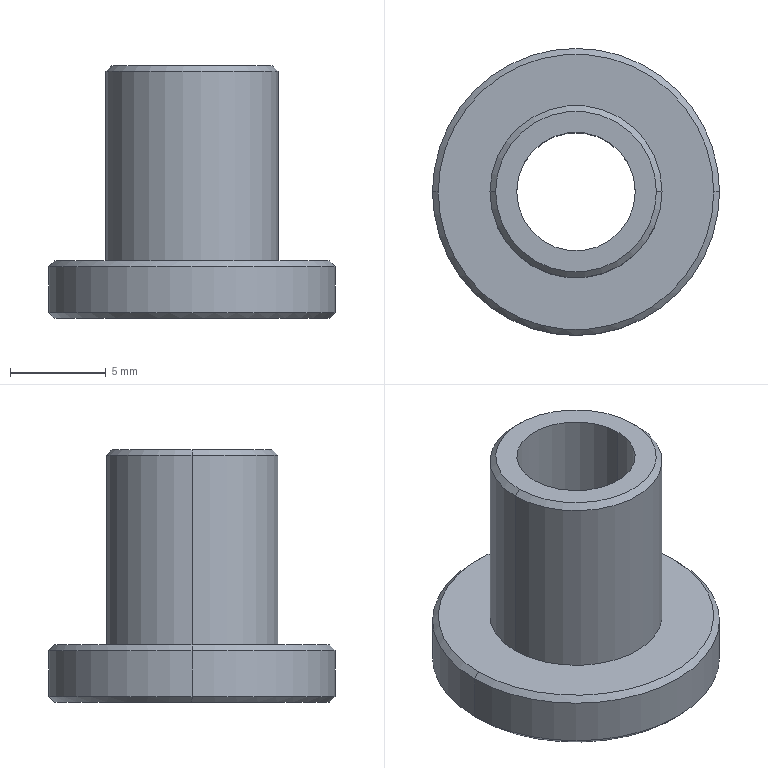Part | STEP file | 1 solid | 15 faces | box 15 x 15 x 13.2 mm | volume 775.094 mm3 | cone 6 | cylinder 6 | plane 3 | commonest cylinder face diameters 6.2 x2 9 x2 15 x2
STEP:
#1=CARTESIAN_POINT('',(0.,0.,0.));
#2=DIRECTION('',(0.,0.,1.));
#3=DIRECTION('',(1.,0.,0.));
#4=AXIS2_PLACEMENT_3D('',#1,#2,#3);
#5=CARTESIAN_POINT('',(-7.2,0.,0.));
#6=VERTEX_POINT('',#5);
#7=CARTESIAN_POINT('',(7.2,0.,0.));
#8=VERTEX_POINT('',#7);
#9=CARTESIAN_POINT('',(0.,0.,0.));
#10=DIRECTION('',(0.,0.,-1.));
#11=DIRECTION('',(1.,0.,0.));
#12=AXIS2_PLACEMENT_3D('',#9,#10,#11);
#13=CIRCLE('',#12,7.2);
#14=CARTESIAN_POINT('',(0.,0.,0.));
#15=DIRECTION('',(0.,0.,1.));
#16=DIRECTION('',(1.,0.,0.));
#17=AXIS2_PLACEMENT_3D('',#14,#15,#16);
#18=CONICAL_SURFACE('',#17,7.2,0.7854);
#19=CARTESIAN_POINT('',(6.283,0.));
#20=DIRECTION('',(-1.,0.));
#21=VECTOR('',#20,1.);
#22=LINE('',#19,#21);
#23=(GEOMETRIC_REPRESENTATION_CONTEXT(2)PARAMETRIC_REPRESENTATION_CONTEXT()REPRESENTATION_CONTEXT('',''));
#24=DEFINITIONAL_REPRESENTATION('',(#22),#23);
#25=PCURVE('',#18,#24);
#26=CARTESIAN_POINT('',(0.,0.,0.));
#27=DIRECTION('',(0.,0.,1.));
#28=DIRECTION('',(1.,0.,0.));
#29=AXIS2_PLACEMENT_3D('',#26,#27,#28);
#30=PLANE('',#29);
#31=CARTESIAN_POINT('',(7.2,0.));
#32=CARTESIAN_POINT('',(7.2,-12.471));
#33=CARTESIAN_POINT('',(-3.6,-6.235));
#34=CARTESIAN_POINT('',(-14.4,0.));
#35=CARTESIAN_POINT('',(-3.6,6.235));
#36=CARTESIAN_POINT('',(7.2,12.471));
#37=CARTESIAN_POINT('',(7.2,0.));
#38=(BOUNDED_CURVE()B_SPLINE_CURVE(2,(#31,#32,#33,#34,#35,#36,#37),.UNSPECIFIED.,.T.,.F.)B_SPLINE_CURVE_WITH_KNOTS((1,2,2,2,2,1),(-2.094,0.,2.094,4.189,6.283,8.378),.UNSPECIFIED.)CURVE()GEOMETRIC_REPRESENTATION_ITEM()RATIONAL_B_SPLINE_CURVE((1.,0.5,1.,0.5,1.,0.5,1.))REPRESENTATION_ITEM(''));
#39=(GEOMETRIC_REPRESENTATION_CONTEXT(2)PARAMETRIC_REPRESENTATION_CONTEXT()REPRESENTATION_CONTEXT('',''));
#40=DEFINITIONAL_REPRESENTATION('',(#38),#39);
#41=PCURVE('',#30,#40);
#42=SURFACE_CURVE('',#13,(#25,#41),.PCURVE_S1.);
#43=EDGE_CURVE('',#6,#8,#42,.T.);
#44=ORIENTED_EDGE('',*,*,#43,.F.);
#45=CARTESIAN_POINT('',(-7.5,0.,0.3));
#46=VERTEX_POINT('',#45);
#47=CARTESIAN_POINT('',(-7.2,0.,0.));
#48=DIRECTION('',(-0.7071,0.,0.7071));
#49=VECTOR('',#48,1.);
#50=LINE('',#47,#49);
#51=CARTESIAN_POINT('',(3.142,0.));
#52=DIRECTION('',(0.,1.));
#53=VECTOR('',#52,1.);
#54=LINE('',#51,#53);
#55=(GEOMETRIC_REPRESENTATION_CONTEXT(2)PARAMETRIC_REPRESENTATION_CONTEXT()REPRESENTATION_CONTEXT('',''));
#56=DEFINITIONAL_REPRESENTATION('',(#54),#55);
#57=PCURVE('',#18,#56);
#58=CARTESIAN_POINT('',(0.,0.,0.));
#59=DIRECTION('',(0.,0.,1.));
#60=DIRECTION('',(1.,0.,0.));
#61=AXIS2_PLACEMENT_3D('',#58,#59,#60);
#62=CONICAL_SURFACE('',#61,7.2,0.7854);
#63=CARTESIAN_POINT('',(3.142,0.));
#64=DIRECTION('',(0.,1.));
#65=VECTOR('',#64,1.);
#66=LINE('',#63,#65);
#67=(GEOMETRIC_REPRESENTATION_CONTEXT(2)PARAMETRIC_REPRESENTATION_CONTEXT()REPRESENTATION_CONTEXT('',''));
#68=DEFINITIONAL_REPRESENTATION('',(#66),#67);
#69=PCURVE('',#62,#68);
#70=SURFACE_CURVE('',#50,(#57,#69),.PCURVE_S1.);
#71=EDGE_CURVE('',#6,#46,#70,.T.);
#72=ORIENTED_EDGE('',*,*,#71,.T.);
#73=CARTESIAN_POINT('',(7.5,0.,0.3));
#74=VERTEX_POINT('',#73);
#75=CARTESIAN_POINT('',(0.,0.,0.3));
#76=DIRECTION('',(0.,0.,1.));
#77=DIRECTION('',(1.,0.,0.));
#78=AXIS2_PLACEMENT_3D('',#75,#76,#77);
#79=CIRCLE('',#78,7.5);
#80=CARTESIAN_POINT('',(0.,0.3));
#81=DIRECTION('',(1.,0.));
#82=VECTOR('',#81,1.);
#83=LINE('',#80,#82);
#84=(GEOMETRIC_REPRESENTATION_CONTEXT(2)PARAMETRIC_REPRESENTATION_CONTEXT()REPRESENTATION_CONTEXT('',''));
#85=DEFINITIONAL_REPRESENTATION('',(#83),#84);
#86=PCURVE('',#18,#85);
#87=CARTESIAN_POINT('',(0.,0.,3.));
#88=DIRECTION('',(0.,0.,-1.));
#89=DIRECTION('',(-1.,0.,0.));
#90=AXIS2_PLACEMENT_3D('',#87,#88,#89);
#91=CYLINDRICAL_SURFACE('',#90,7.5);
#92=CARTESIAN_POINT('',(3.142,2.7));
#93=DIRECTION('',(-1.,0.));
#94=VECTOR('',#93,1.);
#95=LINE('',#92,#94);
#96=(GEOMETRIC_REPRESENTATION_CONTEXT(2)PARAMETRIC_REPRESENTATION_CONTEXT()REPRESENTATION_CONTEXT('',''));
#97=DEFINITIONAL_REPRESENTATION('',(#95),#96);
#98=PCURVE('',#91,#97);
#99=SURFACE_CURVE('',#79,(#86,#98),.PCURVE_S1.);
#100=EDGE_CURVE('',#74,#46,#99,.T.);
#101=ORIENTED_EDGE('',*,*,#100,.F.);
#102=CARTESIAN_POINT('',(7.2,0.,0.));
#103=DIRECTION('',(0.7071,0.,0.7071));
#104=VECTOR('',#103,1.);
#105=LINE('',#102,#104);
#106=CARTESIAN_POINT('',(0.,0.));
#107=DIRECTION('',(0.,1.));
#108=VECTOR('',#107,1.);
#109=LINE('',#106,#108);
#110=(GEOMETRIC_REPRESENTATION_CONTEXT(2)PARAMETRIC_REPRESENTATION_CONTEXT()REPRESENTATION_CONTEXT('',''));
#111=DEFINITIONAL_REPRESENTATION('',(#109),#110);
#112=PCURVE('',#18,#111);
#113=CARTESIAN_POINT('',(6.283,0.));
#114=DIRECTION('',(0.,1.));
#115=VECTOR('',#114,1.);
#116=LINE('',#113,#115);
#117=(GEOMETRIC_REPRESENTATION_CONTEXT(2)PARAMETRIC_REPRESENTATION_CONTEXT()REPRESENTATION_CONTEXT('',''));
#118=DEFINITIONAL_REPRESENTATION('',(#116),#117);
#119=PCURVE('',#62,#118);
#120=SURFACE_CURVE('',#105,(#112,#119),.PCURVE_S1.);
#121=EDGE_CURVE('',#8,#74,#120,.T.);
#122=ORIENTED_EDGE('',*,*,#121,.F.);
#123=EDGE_LOOP('',(#44,#72,#101,#122));
#124=FACE_BOUND('',#123,.T.);
#125=ADVANCED_FACE('',(#124),#18,.T.);
#126=CARTESIAN_POINT('',(7.2,0.,3.));
#127=VERTEX_POINT('',#126);
#128=CARTESIAN_POINT('',(-7.2,0.,3.));
#129=VERTEX_POINT('',#128);
#130=CARTESIAN_POINT('',(0.,0.,3.));
#131=DIRECTION('',(0.,0.,1.));
#132=DIRECTION('',(-1.,0.,0.));
#133=AXIS2_PLACEMENT_3D('',#130,#131,#132);
#134=CIRCLE('',#133,7.2);
#135=CARTESIAN_POINT('',(0.,0.,2.7));
#136=DIRECTION('',(0.,0.,-1.));
#137=DIRECTION('',(-1.,0.,0.));
#138=AXIS2_PLACEMENT_3D('',#135,#136,#137);
#139=CONICAL_SURFACE('',#138,7.5,0.7854);
#140=CARTESIAN_POINT('',(6.283,-0.3));
#141=DIRECTION('',(-1.,0.));
#142=VECTOR('',#141,1.);
#143=LINE('',#140,#142);
#144=(GEOMETRIC_REPRESENTATION_CONTEXT(2)PARAMETRIC_REPRESENTATION_CONTEXT()REPRESENTATION_CONTEXT('',''));
#145=DEFINITIONAL_REPRESENTATION('',(#143),#144);
#146=PCURVE('',#139,#145);
#147=CARTESIAN_POINT('',(0.,0.,3.));
#148=DIRECTION('',(0.,0.,-1.));
#149=DIRECTION('',(-1.,0.,0.));
#150=AXIS2_PLACEMENT_3D('',#147,#148,#149);
#151=PLANE('',#150);
#152=CARTESIAN_POINT('',(7.2,0.));
#153=CARTESIAN_POINT('',(7.2,-12.471));
#154=CARTESIAN_POINT('',(-3.6,-6.235));
#155=CARTESIAN_POINT('',(-14.4,0.));
#156=CARTESIAN_POINT('',(-3.6,6.235));
#157=CARTESIAN_POINT('',(7.2,12.471));
#158=CARTESIAN_POINT('',(7.2,0.));
#159=(BOUNDED_CURVE()B_SPLINE_CURVE(2,(#152,#153,#154,#155,#156,#157,#158),.UNSPECIFIED.,.T.,.F.)B_SPLINE_CURVE_WITH_KNOTS((1,2,2,2,2,1),(-2.094,0.,2.094,4.189,6.283,8.378),.UNSPECIFIED.)CURVE()GEOMETRIC_REPRESENTATION_ITEM()RATIONAL_B_SPLINE_CURVE((1.,0.5,1.,0.5,1.,0.5,1.))REPRESENTATION_ITEM(''));
#160=(GEOMETRIC_REPRESENTATION_CONTEXT(2)PARAMETRIC_REPRESENTATION_CONTEXT()REPRESENTATION_CONTEXT('',''));
#161=DEFINITIONAL_REPRESENTATION('',(#159),#160);
#162=PCURVE('',#151,#161);
#163=SURFACE_CURVE('',#134,(#146,#162),.PCURVE_S1.);
#164=EDGE_CURVE('',#127,#129,#163,.T.);
#165=ORIENTED_EDGE('',*,*,#164,.F.);
#166=CARTESIAN_POINT('',(7.5,0.,2.7));
#167=VERTEX_POINT('',#166);
#168=CARTESIAN_POINT('',(7.5,0.,2.7));
#169=DIRECTION('',(0.7071,0.,-0.7071));
#170=VECTOR('',#169,1.);
#171=LINE('',#168,#170);
#172=CARTESIAN_POINT('',(3.142,0.));
#173=DIRECTION('',(0.,1.));
#174=VECTOR('',#173,1.);
#175=LINE('',#172,#174);
#176=(GEOMETRIC_REPRESENTATION_CONTEXT(2)PARAMETRIC_REPRESENTATION_CONTEXT()REPRESENTATION_CONTEXT('',''));
#177=DEFINITIONAL_REPRESENTATION('',(#175),#176);
#178=PCURVE('',#139,#177);
#179=CARTESIAN_POINT('',(0.,0.,2.7));
#180=DIRECTION('',(0.,0.,-1.));
#181=DIRECTION('',(-1.,0.,0.));
#182=AXIS2_PLACEMENT_3D('',#179,#180,#181);
#183=CONICAL_SURFACE('',#182,7.5,0.7854);
#184=CARTESIAN_POINT('',(3.142,0.));
#185=DIRECTION('',(0.,1.));
#186=VECTOR('',#185,1.);
#187=LINE('',#184,#186);
#188=(GEOMETRIC_REPRESENTATION_CONTEXT(2)PARAMETRIC_REPRESENTATION_CONTEXT()REPRESENTATION_CONTEXT('',''));
#189=DEFINITIONAL_REPRESENTATION('',(#187),#188);
#190=PCURVE('',#183,#189);
#191=SURFACE_CURVE('',#171,(#178,#190),.PCURVE_S1.);
#192=EDGE_CURVE('',#127,#167,#191,.T.);
#193=ORIENTED_EDGE('',*,*,#192,.T.);
#194=CARTESIAN_POINT('',(-7.5,0.,2.7));
#195=VERTEX_POINT('',#194);
#196=CARTESIAN_POINT('',(0.,0.,2.7));
#197=DIRECTION('',(0.,0.,-1.));
#198=DIRECTION('',(-1.,0.,0.));
#199=AXIS2_PLACEMENT_3D('',#196,#197,#198);
#200=CIRCLE('',#199,7.5);
#201=CARTESIAN_POINT('',(0.,0.));
#202=DIRECTION('',(1.,0.));
#203=VECTOR('',#202,1.);
#204=LINE('',#201,#203);
#205=(GEOMETRIC_REPRESENTATION_CONTEXT(2)PARAMETRIC_REPRESENTATION_CONTEXT()REPRESENTATION_CONTEXT('',''));
#206=DEFINITIONAL_REPRESENTATION('',(#204),#205);
#207=PCURVE('',#139,#206);
#208=CARTESIAN_POINT('',(0.,0.3));
#209=DIRECTION('',(1.,0.));
#210=VECTOR('',#209,1.);
#211=LINE('',#208,#210);
#212=(GEOMETRIC_REPRESENTATION_CONTEXT(2)PARAMETRIC_REPRESENTATION_CONTEXT()REPRESENTATION_CONTEXT('',''));
#213=DEFINITIONAL_REPRESENTATION('',(#211),#212);
#214=PCURVE('',#91,#213);
#215=SURFACE_CURVE('',#200,(#207,#214),.PCURVE_S1.);
#216=EDGE_CURVE('',#195,#167,#215,.T.);
#217=ORIENTED_EDGE('',*,*,#216,.F.);
#218=CARTESIAN_POINT('',(-7.5,0.,2.7));
#219=DIRECTION('',(-0.7071,0.,-0.7071));
#220=VECTOR('',#219,1.);
#221=LINE('',#218,#220);
#222=CARTESIAN_POINT('',(0.,0.));
#223=DIRECTION('',(0.,1.));
#224=VECTOR('',#223,1.);
#225=LINE('',#222,#224);
#226=(GEOMETRIC_REPRESENTATION_CONTEXT(2)PARAMETRIC_REPRESENTATION_CONTEXT()REPRESENTATION_CONTEXT('',''));
#227=DEFINITIONAL_REPRESENTATION('',(#225),#226);
#228=PCURVE('',#139,#227);
#229=CARTESIAN_POINT('',(6.283,0.));
#230=DIRECTION('',(0.,1.));
#231=VECTOR('',#230,1.);
#232=LINE('',#229,#231);
#233=(GEOMETRIC_REPRESENTATION_CONTEXT(2)PARAMETRIC_REPRESENTATION_CONTEXT()REPRESENTATION_CONTEXT('',''));
#234=DEFINITIONAL_REPRESENTATION('',(#232),#233);
#235=PCURVE('',#183,#234);
#236=SURFACE_CURVE('',#221,(#228,#235),.PCURVE_S1.);
#237=EDGE_CURVE('',#129,#195,#236,.T.);
#238=ORIENTED_EDGE('',*,*,#237,.F.);
#239=EDGE_LOOP('',(#165,#193,#217,#238));
#240=FACE_BOUND('',#239,.T.);
#241=ADVANCED_FACE('',(#240),#139,.T.);
#242=CARTESIAN_POINT('',(4.2,0.,13.2));
#243=VERTEX_POINT('',#242);
#244=CARTESIAN_POINT('',(-4.2,0.,13.2));
#245=VERTEX_POINT('',#244);
#246=CARTESIAN_POINT('',(0.,0.,13.2));
#247=DIRECTION('',(0.,0.,1.));
#248=DIRECTION('',(1.,0.,0.));
#249=AXIS2_PLACEMENT_3D('',#246,#247,#248);
#250=CIRCLE('',#249,4.2);
#251=CARTESIAN_POINT('',(0.,0.,13.2));
#252=DIRECTION('',(0.,0.,-1.));
#253=DIRECTION('',(-1.,0.,0.));
#254=AXIS2_PLACEMENT_3D('',#251,#252,#253);
#255=CONICAL_SURFACE('',#254,4.2,0.7854);
#256=CARTESIAN_POINT('',(3.142,0.));
#257=DIRECTION('',(-1.,0.));
#258=VECTOR('',#257,1.);
#259=LINE('',#256,#258);
#260=(GEOMETRIC_REPRESENTATION_CONTEXT(2)PARAMETRIC_REPRESENTATION_CONTEXT()REPRESENTATION_CONTEXT('',''));
#261=DEFINITIONAL_REPRESENTATION('',(#259),#260);
#262=PCURVE('',#255,#261);
#263=CARTESIAN_POINT('',(0.,0.,13.2));
#264=DIRECTION('',(0.,0.,1.));
#265=DIRECTION('',(1.,0.,0.));
#266=AXIS2_PLACEMENT_3D('',#263,#264,#265);
#267=PLANE('',#266);
#268=CARTESIAN_POINT('',(0.,0.));
#269=DIRECTION('',(1.,0.));
#270=AXIS2_PLACEMENT_2D('',#268,#269);
#271=CIRCLE('',#270,4.2);
#272=(GEOMETRIC_REPRESENTATION_CONTEXT(2)PARAMETRIC_REPRESENTATION_CONTEXT()REPRESENTATION_CONTEXT('',''));
#273=DEFINITIONAL_REPRESENTATION('',(#271),#272);
#274=PCURVE('',#267,#273);
#275=SURFACE_CURVE('',#250,(#262,#274),.PCURVE_S1.);
#276=EDGE_CURVE('',#243,#245,#275,.T.);
#277=ORIENTED_EDGE('',*,*,#276,.F.);
#278=CARTESIAN_POINT('',(4.5,0.,12.9));
#279=VERTEX_POINT('',#278);
#280=CARTESIAN_POINT('',(4.2,0.,13.2));
#281=DIRECTION('',(0.7071,0.,-0.7071));
#282=VECTOR('',#281,1.);
#283=LINE('',#280,#282);
#284=CARTESIAN_POINT('',(3.142,0.));
#285=DIRECTION('',(0.,1.));
#286=VECTOR('',#285,1.);
#287=LINE('',#284,#286);
#288=(GEOMETRIC_REPRESENTATION_CONTEXT(2)PARAMETRIC_REPRESENTATION_CONTEXT()REPRESENTATION_CONTEXT('',''));
#289=DEFINITIONAL_REPRESENTATION('',(#287),#288);
#290=PCURVE('',#255,#289);
#291=CARTESIAN_POINT('',(0.,0.,13.2));
#292=DIRECTION('',(0.,0.,-1.));
#293=DIRECTION('',(-1.,0.,0.));
#294=AXIS2_PLACEMENT_3D('',#291,#292,#293);
#295=CONICAL_SURFACE('',#294,4.2,0.7854);
#296=CARTESIAN_POINT('',(3.142,0.));
#297=DIRECTION('',(0.,1.));
#298=VECTOR('',#297,1.);
#299=LINE('',#296,#298);
#300=(GEOMETRIC_REPRESENTATION_CONTEXT(2)PARAMETRIC_REPRESENTATION_CONTEXT()REPRESENTATION_CONTEXT('',''));
#301=DEFINITIONAL_REPRESENTATION('',(#299),#300);
#302=PCURVE('',#295,#301);
#303=SURFACE_CURVE('',#283,(#290,#302),.PCURVE_S1.);
#304=EDGE_CURVE('',#243,#279,#303,.T.);
#305=ORIENTED_EDGE('',*,*,#304,.T.);
#306=CARTESIAN_POINT('',(-4.5,0.,12.9));
#307=VERTEX_POINT('',#306);
#308=CARTESIAN_POINT('',(0.,0.,12.9));
#309=DIRECTION('',(0.,0.,-1.));
#310=DIRECTION('',(1.,0.,0.));
#311=AXIS2_PLACEMENT_3D('',#308,#309,#310);
#312=CIRCLE('',#311,4.5);
#313=CARTESIAN_POINT('',(-3.142,0.3));
#314=DIRECTION('',(1.,0.));
#315=VECTOR('',#314,1.);
#316=LINE('',#313,#315);
#317=(GEOMETRIC_REPRESENTATION_CONTEXT(2)PARAMETRIC_REPRESENTATION_CONTEXT()REPRESENTATION_CONTEXT('',''));
#318=DEFINITIONAL_REPRESENTATION('',(#316),#317);
#319=PCURVE('',#255,#318);
#320=CARTESIAN_POINT('',(0.,0.,13.2));
#321=DIRECTION('',(0.,0.,-1.));
#322=DIRECTION('',(-1.,0.,0.));
#323=AXIS2_PLACEMENT_3D('',#320,#321,#322);
#324=CYLINDRICAL_SURFACE('',#323,4.5);
#325=CARTESIAN_POINT('',(-3.142,0.3));
#326=DIRECTION('',(1.,0.));
#327=VECTOR('',#326,1.);
#328=LINE('',#325,#327);
#329=(GEOMETRIC_REPRESENTATION_CONTEXT(2)PARAMETRIC_REPRESENTATION_CONTEXT()REPRESENTATION_CONTEXT('',''));
#330=DEFINITIONAL_REPRESENTATION('',(#328),#329);
#331=PCURVE('',#324,#330);
#332=SURFACE_CURVE('',#312,(#319,#331),.PCURVE_S1.);
#333=EDGE_CURVE('',#307,#279,#332,.T.);
#334=ORIENTED_EDGE('',*,*,#333,.F.);
#335=CARTESIAN_POINT('',(-4.2,0.,13.2));
#336=DIRECTION('',(-0.7071,0.,-0.7071));
#337=VECTOR('',#336,1.);
#338=LINE('',#335,#337);
#339=CARTESIAN_POINT('',(0.,0.));
#340=DIRECTION('',(0.,1.));
#341=VECTOR('',#340,1.);
#342=LINE('',#339,#341);
#343=(GEOMETRIC_REPRESENTATION_CONTEXT(2)PARAMETRIC_REPRESENTATION_CONTEXT()REPRESENTATION_CONTEXT('',''));
#344=DEFINITIONAL_REPRESENTATION('',(#342),#343);
#345=PCURVE('',#255,#344);
#346=CARTESIAN_POINT('',(6.283,0.));
#347=DIRECTION('',(0.,1.));
#348=VECTOR('',#347,1.);
#349=LINE('',#346,#348);
#350=(GEOMETRIC_REPRESENTATION_CONTEXT(2)PARAMETRIC_REPRESENTATION_CONTEXT()REPRESENTATION_CONTEXT('',''));
#351=DEFINITIONAL_REPRESENTATION('',(#349),#350);
#352=PCURVE('',#295,#351);
#353=SURFACE_CURVE('',#338,(#345,#352),.PCURVE_S1.);
#354=EDGE_CURVE('',#245,#307,#353,.T.);
#355=ORIENTED_EDGE('',*,*,#354,.F.);
#356=EDGE_LOOP('',(#277,#305,#334,#355));
#357=FACE_BOUND('',#356,.T.);
#358=ADVANCED_FACE('',(#357),#255,.T.);
#359=ORIENTED_EDGE('',*,*,#216,.T.);
#360=CARTESIAN_POINT('',(7.5,0.,3.));
#361=DIRECTION('',(0.,0.,-1.));
#362=VECTOR('',#361,1.);
#363=LINE('',#360,#362);
#364=CARTESIAN_POINT('',(3.142,0.));
#365=DIRECTION('',(0.,1.));
#366=VECTOR('',#365,1.);
#367=LINE('',#364,#366);
#368=(GEOMETRIC_REPRESENTATION_CONTEXT(2)PARAMETRIC_REPRESENTATION_CONTEXT()REPRESENTATION_CONTEXT('',''));
#369=DEFINITIONAL_REPRESENTATION('',(#367),#368);
#370=PCURVE('',#91,#369);
#371=CARTESIAN_POINT('',(0.,0.,3.));
#372=DIRECTION('',(0.,0.,-1.));
#373=DIRECTION('',(-1.,0.,0.));
#374=AXIS2_PLACEMENT_3D('',#371,#372,#373);
#375=CYLINDRICAL_SURFACE('',#374,7.5);
#376=CARTESIAN_POINT('',(3.142,0.));
#377=DIRECTION('',(0.,1.));
#378=VECTOR('',#377,1.);
#379=LINE('',#376,#378);
#380=(GEOMETRIC_REPRESENTATION_CONTEXT(2)PARAMETRIC_REPRESENTATION_CONTEXT()REPRESENTATION_CONTEXT('',''));
#381=DEFINITIONAL_REPRESENTATION('',(#379),#380);
#382=PCURVE('',#375,#381);
#383=SURFACE_CURVE('',#363,(#370,#382),.PCURVE_S1.);
#384=EDGE_CURVE('',#167,#74,#383,.T.);
#385=ORIENTED_EDGE('',*,*,#384,.T.);
#386=ORIENTED_EDGE('',*,*,#100,.T.);
#387=CARTESIAN_POINT('',(-7.5,0.,3.));
#388=DIRECTION('',(0.,0.,-1.));
#389=VECTOR('',#388,1.);
#390=LINE('',#387,#389);
#391=CARTESIAN_POINT('',(0.,0.));
#392=DIRECTION('',(0.,1.));
#393=VECTOR('',#392,1.);
#394=LINE('',#391,#393);
#395=(GEOMETRIC_REPRESENTATION_CONTEXT(2)PARAMETRIC_REPRESENTATION_CONTEXT()REPRESENTATION_CONTEXT('',''));
#396=DEFINITIONAL_REPRESENTATION('',(#394),#395);
#397=PCURVE('',#91,#396);
#398=CARTESIAN_POINT('',(6.283,0.));
#399=DIRECTION('',(0.,1.));
#400=VECTOR('',#399,1.);
#401=LINE('',#398,#400);
#402=(GEOMETRIC_REPRESENTATION_CONTEXT(2)PARAMETRIC_REPRESENTATION_CONTEXT()REPRESENTATION_CONTEXT('',''));
#403=DEFINITIONAL_REPRESENTATION('',(#401),#402);
#404=PCURVE('',#375,#403);
#405=SURFACE_CURVE('',#390,(#397,#404),.PCURVE_S1.);
#406=EDGE_CURVE('',#195,#46,#405,.T.);
#407=ORIENTED_EDGE('',*,*,#406,.F.);
#408=EDGE_LOOP('',(#359,#385,#386,#407));
#409=FACE_BOUND('',#408,.T.);
#410=ADVANCED_FACE('',(#409),#91,.T.);
#411=CARTESIAN_POINT('',(-3.1,0.,13.2));
#412=VERTEX_POINT('',#411);
#413=CARTESIAN_POINT('',(-3.1,0.,0.));
#414=VERTEX_POINT('',#413);
#415=CARTESIAN_POINT('',(-3.1,0.,13.2));
#416=DIRECTION('',(0.,0.,-1.));
#417=VECTOR('',#416,1.);
#418=LINE('',#415,#417);
#419=CARTESIAN_POINT('',(0.,0.,13.2));
#420=DIRECTION('',(0.,0.,-1.));
#421=DIRECTION('',(-1.,0.,0.));
#422=AXIS2_PLACEMENT_3D('',#419,#420,#421);
#423=CYLINDRICAL_SURFACE('',#422,3.1);
#424=CARTESIAN_POINT('',(6.283,0.));
#425=DIRECTION('',(0.,1.));
#426=VECTOR('',#425,1.);
#427=LINE('',#424,#426);
#428=(GEOMETRIC_REPRESENTATION_CONTEXT(2)PARAMETRIC_REPRESENTATION_CONTEXT()REPRESENTATION_CONTEXT('',''));
#429=DEFINITIONAL_REPRESENTATION('',(#427),#428);
#430=PCURVE('',#423,#429);
#431=CARTESIAN_POINT('',(0.,0.,13.2));
#432=DIRECTION('',(0.,0.,-1.));
#433=DIRECTION('',(-1.,0.,0.));
#434=AXIS2_PLACEMENT_3D('',#431,#432,#433);
#435=CYLINDRICAL_SURFACE('',#434,3.1);
#436=CARTESIAN_POINT('',(0.,0.));
#437=DIRECTION('',(0.,1.));
#438=VECTOR('',#437,1.);
#439=LINE('',#436,#438);
#440=(GEOMETRIC_REPRESENTATION_CONTEXT(2)PARAMETRIC_REPRESENTATION_CONTEXT()REPRESENTATION_CONTEXT('',''));
#441=DEFINITIONAL_REPRESENTATION('',(#439),#440);
#442=PCURVE('',#435,#441);
#443=SURFACE_CURVE('',#418,(#430,#442),.PCURVE_S1.);
#444=EDGE_CURVE('',#412,#414,#443,.T.);
#445=ORIENTED_EDGE('',*,*,#444,.T.);
#446=CARTESIAN_POINT('',(3.1,0.,0.));
#447=VERTEX_POINT('',#446);
#448=CARTESIAN_POINT('',(0.,0.,0.));
#449=DIRECTION('',(0.,0.,1.));
#450=DIRECTION('',(1.,0.,0.));
#451=AXIS2_PLACEMENT_3D('',#448,#449,#450);
#452=CIRCLE('',#451,3.1);
#453=CARTESIAN_POINT('',(9.425,13.2));
#454=DIRECTION('',(-1.,0.));
#455=VECTOR('',#454,1.);
#456=LINE('',#453,#455);
#457=(GEOMETRIC_REPRESENTATION_CONTEXT(2)PARAMETRIC_REPRESENTATION_CONTEXT()REPRESENTATION_CONTEXT('',''));
#458=DEFINITIONAL_REPRESENTATION('',(#456),#457);
#459=PCURVE('',#423,#458);
#460=CARTESIAN_POINT('',(0.,0.));
#461=DIRECTION('',(1.,0.));
#462=AXIS2_PLACEMENT_2D('',#460,#461);
#463=CIRCLE('',#462,3.1);
#464=(GEOMETRIC_REPRESENTATION_CONTEXT(2)PARAMETRIC_REPRESENTATION_CONTEXT()REPRESENTATION_CONTEXT('',''));
#465=DEFINITIONAL_REPRESENTATION('',(#463),#464);
#466=PCURVE('',#30,#465);
#467=SURFACE_CURVE('',#452,(#459,#466),.PCURVE_S1.);
#468=EDGE_CURVE('',#414,#447,#467,.T.);
#469=ORIENTED_EDGE('',*,*,#468,.T.);
#470=CARTESIAN_POINT('',(3.1,0.,13.2));
#471=VERTEX_POINT('',#470);
#472=CARTESIAN_POINT('',(3.1,0.,13.2));
#473=DIRECTION('',(0.,0.,-1.));
#474=VECTOR('',#473,1.);
#475=LINE('',#472,#474);
#476=CARTESIAN_POINT('',(3.142,0.));
#477=DIRECTION('',(0.,1.));
#478=VECTOR('',#477,1.);
#479=LINE('',#476,#478);
#480=(GEOMETRIC_REPRESENTATION_CONTEXT(2)PARAMETRIC_REPRESENTATION_CONTEXT()REPRESENTATION_CONTEXT('',''));
#481=DEFINITIONAL_REPRESENTATION('',(#479),#480);
#482=PCURVE('',#423,#481);
#483=CARTESIAN_POINT('',(3.142,0.));
#484=DIRECTION('',(0.,1.));
#485=VECTOR('',#484,1.);
#486=LINE('',#483,#485);
#487=(GEOMETRIC_REPRESENTATION_CONTEXT(2)PARAMETRIC_REPRESENTATION_CONTEXT()REPRESENTATION_CONTEXT('',''));
#488=DEFINITIONAL_REPRESENTATION('',(#486),#487);
#489=PCURVE('',#435,#488);
#490=SURFACE_CURVE('',#475,(#482,#489),.PCURVE_S1.);
#491=EDGE_CURVE('',#471,#447,#490,.T.);
#492=ORIENTED_EDGE('',*,*,#491,.F.);
#493=CARTESIAN_POINT('',(0.,0.,13.2));
#494=DIRECTION('',(0.,0.,1.));
#495=DIRECTION('',(1.,0.,0.));
#496=AXIS2_PLACEMENT_3D('',#493,#494,#495);
#497=CIRCLE('',#496,3.1);
#498=CARTESIAN_POINT('',(9.425,0.));
#499=DIRECTION('',(-1.,0.));
#500=VECTOR('',#499,1.);
#501=LINE('',#498,#500);
#502=(GEOMETRIC_REPRESENTATION_CONTEXT(2)PARAMETRIC_REPRESENTATION_CONTEXT()REPRESENTATION_CONTEXT('',''));
#503=DEFINITIONAL_REPRESENTATION('',(#501),#502);
#504=PCURVE('',#423,#503);
#505=CARTESIAN_POINT('',(0.,0.));
#506=DIRECTION('',(1.,0.));
#507=AXIS2_PLACEMENT_2D('',#505,#506);
#508=CIRCLE('',#507,3.1);
#509=(GEOMETRIC_REPRESENTATION_CONTEXT(2)PARAMETRIC_REPRESENTATION_CONTEXT()REPRESENTATION_CONTEXT('',''));
#510=DEFINITIONAL_REPRESENTATION('',(#508),#509);
#511=PCURVE('',#267,#510);
#512=SURFACE_CURVE('',#497,(#504,#511),.PCURVE_S1.);
#513=EDGE_CURVE('',#412,#471,#512,.T.);
#514=ORIENTED_EDGE('',*,*,#513,.F.);
#515=EDGE_LOOP('',(#445,#469,#492,#514));
#516=FACE_BOUND('',#515,.F.);
#517=ADVANCED_FACE('',(#516),#423,.F.);
#518=ORIENTED_EDGE('',*,*,#333,.T.);
#519=CARTESIAN_POINT('',(4.5,0.,3.));
#520=VERTEX_POINT('',#519);
#521=CARTESIAN_POINT('',(4.5,0.,13.2));
#522=DIRECTION('',(0.,0.,-1.));
#523=VECTOR('',#522,1.);
#524=LINE('',#521,#523);
#525=CARTESIAN_POINT('',(3.142,0.));
#526=DIRECTION('',(0.,1.));
#527=VECTOR('',#526,1.);
#528=LINE('',#525,#527);
#529=(GEOMETRIC_REPRESENTATION_CONTEXT(2)PARAMETRIC_REPRESENTATION_CONTEXT()REPRESENTATION_CONTEXT('',''));
#530=DEFINITIONAL_REPRESENTATION('',(#528),#529);
#531=PCURVE('',#324,#530);
#532=CARTESIAN_POINT('',(0.,0.,13.2));
#533=DIRECTION('',(0.,0.,-1.));
#534=DIRECTION('',(-1.,0.,0.));
#535=AXIS2_PLACEMENT_3D('',#532,#533,#534);
#536=CYLINDRICAL_SURFACE('',#535,4.5);
#537=CARTESIAN_POINT('',(3.142,0.));
#538=DIRECTION('',(0.,1.));
#539=VECTOR('',#538,1.);
#540=LINE('',#537,#539);
#541=(GEOMETRIC_REPRESENTATION_CONTEXT(2)PARAMETRIC_REPRESENTATION_CONTEXT()REPRESENTATION_CONTEXT('',''));
#542=DEFINITIONAL_REPRESENTATION('',(#540),#541);
#543=PCURVE('',#536,#542);
#544=SURFACE_CURVE('',#524,(#531,#543),.PCURVE_S1.);
#545=EDGE_CURVE('',#279,#520,#544,.T.);
#546=ORIENTED_EDGE('',*,*,#545,.T.);
#547=CARTESIAN_POINT('',(-4.5,0.,3.));
#548=VERTEX_POINT('',#547);
#549=CARTESIAN_POINT('',(0.,0.,3.));
#550=DIRECTION('',(0.,0.,-1.));
#551=DIRECTION('',(-1.,0.,0.));
#552=AXIS2_PLACEMENT_3D('',#549,#550,#551);
#553=CIRCLE('',#552,4.5);
#554=CARTESIAN_POINT('',(0.,10.2));
#555=DIRECTION('',(1.,0.));
#556=VECTOR('',#555,1.);
#557=LINE('',#554,#556);
#558=(GEOMETRIC_REPRESENTATION_CONTEXT(2)PARAMETRIC_REPRESENTATION_CONTEXT()REPRESENTATION_CONTEXT('',''));
#559=DEFINITIONAL_REPRESENTATION('',(#557),#558);
#560=PCURVE('',#324,#559);
#561=CARTESIAN_POINT('',(0.,0.));
#562=DIRECTION('',(1.,0.));
#563=AXIS2_PLACEMENT_2D('',#561,#562);
#564=CIRCLE('',#563,4.5);
#565=(GEOMETRIC_REPRESENTATION_CONTEXT(2)PARAMETRIC_REPRESENTATION_CONTEXT()REPRESENTATION_CONTEXT('',''));
#566=DEFINITIONAL_REPRESENTATION('',(#564),#565);
#567=PCURVE('',#151,#566);
#568=SURFACE_CURVE('',#553,(#560,#567),.PCURVE_S1.);
#569=EDGE_CURVE('',#548,#520,#568,.T.);
#570=ORIENTED_EDGE('',*,*,#569,.F.);
#571=CARTESIAN_POINT('',(-4.5,0.,13.2));
#572=DIRECTION('',(0.,0.,-1.));
#573=VECTOR('',#572,1.);
#574=LINE('',#571,#573);
#575=CARTESIAN_POINT('',(0.,0.));
#576=DIRECTION('',(0.,1.));
#577=VECTOR('',#576,1.);
#578=LINE('',#575,#577);
#579=(GEOMETRIC_REPRESENTATION_CONTEXT(2)PARAMETRIC_REPRESENTATION_CONTEXT()REPRESENTATION_CONTEXT('',''));
#580=DEFINITIONAL_REPRESENTATION('',(#578),#579);
#581=PCURVE('',#324,#580);
#582=CARTESIAN_POINT('',(6.283,0.));
#583=DIRECTION('',(0.,1.));
#584=VECTOR('',#583,1.);
#585=LINE('',#582,#584);
#586=(GEOMETRIC_REPRESENTATION_CONTEXT(2)PARAMETRIC_REPRESENTATION_CONTEXT()REPRESENTATION_CONTEXT('',''));
#587=DEFINITIONAL_REPRESENTATION('',(#585),#586);
#588=PCURVE('',#536,#587);
#589=SURFACE_CURVE('',#574,(#581,#588),.PCURVE_S1.);
#590=EDGE_CURVE('',#307,#548,#589,.T.);
#591=ORIENTED_EDGE('',*,*,#590,.F.);
#592=EDGE_LOOP('',(#518,#546,#570,#591));
#593=FACE_BOUND('',#592,.T.);
#594=ADVANCED_FACE('',(#593),#324,.T.);
#595=ORIENTED_EDGE('',*,*,#545,.F.);
#596=CARTESIAN_POINT('',(0.,0.,12.9));
#597=DIRECTION('',(0.,0.,-1.));
#598=DIRECTION('',(1.,0.,0.));
#599=AXIS2_PLACEMENT_3D('',#596,#597,#598);
#600=CIRCLE('',#599,4.5);
#601=CARTESIAN_POINT('',(3.142,0.3));
#602=DIRECTION('',(1.,0.));
#603=VECTOR('',#602,1.);
#604=LINE('',#601,#603);
#605=(GEOMETRIC_REPRESENTATION_CONTEXT(2)PARAMETRIC_REPRESENTATION_CONTEXT()REPRESENTATION_CONTEXT('',''));
#606=DEFINITIONAL_REPRESENTATION('',(#604),#605);
#607=PCURVE('',#536,#606);
#608=CARTESIAN_POINT('',(3.142,0.3));
#609=DIRECTION('',(1.,0.));
#610=VECTOR('',#609,1.);
#611=LINE('',#608,#610);
#612=(GEOMETRIC_REPRESENTATION_CONTEXT(2)PARAMETRIC_REPRESENTATION_CONTEXT()REPRESENTATION_CONTEXT('',''));
#613=DEFINITIONAL_REPRESENTATION('',(#611),#612);
#614=PCURVE('',#295,#613);
#615=SURFACE_CURVE('',#600,(#607,#614),.PCURVE_S1.);
#616=EDGE_CURVE('',#279,#307,#615,.T.);
#617=ORIENTED_EDGE('',*,*,#616,.T.);
#618=ORIENTED_EDGE('',*,*,#590,.T.);
#619=CARTESIAN_POINT('',(0.,0.,3.));
#620=DIRECTION('',(0.,0.,-1.));
#621=DIRECTION('',(-1.,0.,0.));
#622=AXIS2_PLACEMENT_3D('',#619,#620,#621);
#623=CIRCLE('',#622,4.5);
#624=CARTESIAN_POINT('',(0.,10.2));
#625=DIRECTION('',(1.,0.));
#626=VECTOR('',#625,1.);
#627=LINE('',#624,#626);
#628=(GEOMETRIC_REPRESENTATION_CONTEXT(2)PARAMETRIC_REPRESENTATION_CONTEXT()REPRESENTATION_CONTEXT('',''));
#629=DEFINITIONAL_REPRESENTATION('',(#627),#628);
#630=PCURVE('',#536,#629);
#631=CARTESIAN_POINT('',(0.,0.));
#632=DIRECTION('',(1.,0.));
#633=AXIS2_PLACEMENT_2D('',#631,#632);
#634=CIRCLE('',#633,4.5);
#635=(GEOMETRIC_REPRESENTATION_CONTEXT(2)PARAMETRIC_REPRESENTATION_CONTEXT()REPRESENTATION_CONTEXT('',''));
#636=DEFINITIONAL_REPRESENTATION('',(#634),#635);
#637=PCURVE('',#151,#636);
#638=SURFACE_CURVE('',#623,(#630,#637),.PCURVE_S1.);
#639=EDGE_CURVE('',#520,#548,#638,.T.);
#640=ORIENTED_EDGE('',*,*,#639,.F.);
#641=EDGE_LOOP('',(#595,#617,#618,#640));
#642=FACE_BOUND('',#641,.T.);
#643=ADVANCED_FACE('',(#642),#536,.T.);
#644=CARTESIAN_POINT('',(0.,0.,13.2));
#645=DIRECTION('',(0.,0.,1.));
#646=DIRECTION('',(1.,0.,0.));
#647=AXIS2_PLACEMENT_3D('',#644,#645,#646);
#648=CIRCLE('',#647,4.2);
#649=CARTESIAN_POINT('',(0.,0.));
#650=DIRECTION('',(1.,0.));
#651=AXIS2_PLACEMENT_2D('',#649,#650);
#652=CIRCLE('',#651,4.2);
#653=(GEOMETRIC_REPRESENTATION_CONTEXT(2)PARAMETRIC_REPRESENTATION_CONTEXT()REPRESENTATION_CONTEXT('',''));
#654=DEFINITIONAL_REPRESENTATION('',(#652),#653);
#655=PCURVE('',#267,#654);
#656=CARTESIAN_POINT('',(9.425,0.));
#657=DIRECTION('',(-1.,0.));
#658=VECTOR('',#657,1.);
#659=LINE('',#656,#658);
#660=(GEOMETRIC_REPRESENTATION_CONTEXT(2)PARAMETRIC_REPRESENTATION_CONTEXT()REPRESENTATION_CONTEXT('',''));
#661=DEFINITIONAL_REPRESENTATION('',(#659),#660);
#662=PCURVE('',#295,#661);
#663=SURFACE_CURVE('',#648,(#655,#662),.PCURVE_S1.);
#664=EDGE_CURVE('',#245,#243,#663,.T.);
#665=ORIENTED_EDGE('',*,*,#664,.T.);
#666=ORIENTED_EDGE('',*,*,#276,.T.);
#667=EDGE_LOOP('',(#665,#666));
#668=FACE_BOUND('',#667,.T.);
#669=ORIENTED_EDGE('',*,*,#513,.F.);
#670=CARTESIAN_POINT('',(0.,0.,13.2));
#671=DIRECTION('',(0.,0.,1.));
#672=DIRECTION('',(1.,0.,0.));
#673=AXIS2_PLACEMENT_3D('',#670,#671,#672);
#674=CIRCLE('',#673,3.1);
#675=CARTESIAN_POINT('',(0.,0.));
#676=DIRECTION('',(1.,0.));
#677=AXIS2_PLACEMENT_2D('',#675,#676);
#678=CIRCLE('',#677,3.1);
#679=(GEOMETRIC_REPRESENTATION_CONTEXT(2)PARAMETRIC_REPRESENTATION_CONTEXT()REPRESENTATION_CONTEXT('',''));
#680=DEFINITIONAL_REPRESENTATION('',(#678),#679);
#681=PCURVE('',#267,#680);
#682=CARTESIAN_POINT('',(3.142,0.));
#683=DIRECTION('',(-1.,0.));
#684=VECTOR('',#683,1.);
#685=LINE('',#682,#684);
#686=(GEOMETRIC_REPRESENTATION_CONTEXT(2)PARAMETRIC_REPRESENTATION_CONTEXT()REPRESENTATION_CONTEXT('',''));
#687=DEFINITIONAL_REPRESENTATION('',(#685),#686);
#688=PCURVE('',#435,#687);
#689=SURFACE_CURVE('',#674,(#681,#688),.PCURVE_S1.);
#690=EDGE_CURVE('',#471,#412,#689,.T.);
#691=ORIENTED_EDGE('',*,*,#690,.F.);
#692=EDGE_LOOP('',(#669,#691));
#693=FACE_BOUND('',#692,.T.);
#694=ADVANCED_FACE('',(#668,#693),#267,.T.);
#695=CARTESIAN_POINT('',(0.,0.,0.));
#696=DIRECTION('',(0.,0.,-1.));
#697=DIRECTION('',(1.,0.,0.));
#698=AXIS2_PLACEMENT_3D('',#695,#696,#697);
#699=CIRCLE('',#698,7.2);
#700=CARTESIAN_POINT('',(7.2,0.));
#701=CARTESIAN_POINT('',(7.2,-12.471));
#702=CARTESIAN_POINT('',(-3.6,-6.235));
#703=CARTESIAN_POINT('',(-14.4,0.));
#704=CARTESIAN_POINT('',(-3.6,6.235));
#705=CARTESIAN_POINT('',(7.2,12.471));
#706=CARTESIAN_POINT('',(7.2,0.));
#707=(BOUNDED_CURVE()B_SPLINE_CURVE(2,(#700,#701,#702,#703,#704,#705,#706),.UNSPECIFIED.,.T.,.F.)B_SPLINE_CURVE_WITH_KNOTS((1,2,2,2,2,1),(-2.094,0.,2.094,4.189,6.283,8.378),.UNSPECIFIED.)CURVE()GEOMETRIC_REPRESENTATION_ITEM()RATIONAL_B_SPLINE_CURVE((1.,0.5,1.,0.5,1.,0.5,1.))REPRESENTATION_ITEM(''));
#708=(GEOMETRIC_REPRESENTATION_CONTEXT(2)PARAMETRIC_REPRESENTATION_CONTEXT()REPRESENTATION_CONTEXT('',''));
#709=DEFINITIONAL_REPRESENTATION('',(#707),#708);
#710=PCURVE('',#30,#709);
#711=CARTESIAN_POINT('',(6.283,0.));
#712=DIRECTION('',(-1.,0.));
#713=VECTOR('',#712,1.);
#714=LINE('',#711,#713);
#715=(GEOMETRIC_REPRESENTATION_CONTEXT(2)PARAMETRIC_REPRESENTATION_CONTEXT()REPRESENTATION_CONTEXT('',''));
#716=DEFINITIONAL_REPRESENTATION('',(#714),#715);
#717=PCURVE('',#62,#716);
#718=SURFACE_CURVE('',#699,(#710,#717),.PCURVE_S1.);
#719=EDGE_CURVE('',#8,#6,#718,.T.);
#720=ORIENTED_EDGE('',*,*,#719,.T.);
#721=ORIENTED_EDGE('',*,*,#43,.T.);
#722=EDGE_LOOP('',(#720,#721));
#723=FACE_BOUND('',#722,.T.);
#724=ORIENTED_EDGE('',*,*,#468,.T.);
#725=CARTESIAN_POINT('',(0.,0.,0.));
#726=DIRECTION('',(0.,0.,1.));
#727=DIRECTION('',(1.,0.,0.));
#728=AXIS2_PLACEMENT_3D('',#725,#726,#727);
#729=CIRCLE('',#728,3.1);
#730=CARTESIAN_POINT('',(0.,0.));
#731=DIRECTION('',(1.,0.));
#732=AXIS2_PLACEMENT_2D('',#730,#731);
#733=CIRCLE('',#732,3.1);
#734=(GEOMETRIC_REPRESENTATION_CONTEXT(2)PARAMETRIC_REPRESENTATION_CONTEXT()REPRESENTATION_CONTEXT('',''));
#735=DEFINITIONAL_REPRESENTATION('',(#733),#734);
#736=PCURVE('',#30,#735);
#737=CARTESIAN_POINT('',(3.142,13.2));
#738=DIRECTION('',(-1.,0.));
#739=VECTOR('',#738,1.);
#740=LINE('',#737,#739);
#741=(GEOMETRIC_REPRESENTATION_CONTEXT(2)PARAMETRIC_REPRESENTATION_CONTEXT()REPRESENTATION_CONTEXT('',''));
#742=DEFINITIONAL_REPRESENTATION('',(#740),#741);
#743=PCURVE('',#435,#742);
#744=SURFACE_CURVE('',#729,(#736,#743),.PCURVE_S1.);
#745=EDGE_CURVE('',#447,#414,#744,.T.);
#746=ORIENTED_EDGE('',*,*,#745,.T.);
#747=EDGE_LOOP('',(#724,#746));
#748=FACE_BOUND('',#747,.T.);
#749=ADVANCED_FACE('',(#723,#748),#30,.F.);
#750=ORIENTED_EDGE('',*,*,#745,.T.);
#751=ORIENTED_EDGE('',*,*,#444,.F.);
#752=ORIENTED_EDGE('',*,*,#690,.F.);
#753=ORIENTED_EDGE('',*,*,#491,.T.);
#754=EDGE_LOOP('',(#750,#751,#752,#753));
#755=FACE_BOUND('',#754,.F.);
#756=ADVANCED_FACE('',(#755),#435,.F.);
#757=ORIENTED_EDGE('',*,*,#384,.F.);
#758=CARTESIAN_POINT('',(0.,0.,2.7));
#759=DIRECTION('',(0.,0.,-1.));
#760=DIRECTION('',(-1.,0.,0.));
#761=AXIS2_PLACEMENT_3D('',#758,#759,#760);
#762=CIRCLE('',#761,7.5);
#763=CARTESIAN_POINT('',(0.,0.3));
#764=DIRECTION('',(1.,0.));
#765=VECTOR('',#764,1.);
#766=LINE('',#763,#765);
#767=(GEOMETRIC_REPRESENTATION_CONTEXT(2)PARAMETRIC_REPRESENTATION_CONTEXT()REPRESENTATION_CONTEXT('',''));
#768=DEFINITIONAL_REPRESENTATION('',(#766),#767);
#769=PCURVE('',#375,#768);
#770=CARTESIAN_POINT('',(0.,0.));
#771=DIRECTION('',(1.,0.));
#772=VECTOR('',#771,1.);
#773=LINE('',#770,#772);
#774=(GEOMETRIC_REPRESENTATION_CONTEXT(2)PARAMETRIC_REPRESENTATION_CONTEXT()REPRESENTATION_CONTEXT('',''));
#775=DEFINITIONAL_REPRESENTATION('',(#773),#774);
#776=PCURVE('',#183,#775);
#777=SURFACE_CURVE('',#762,(#769,#776),.PCURVE_S1.);
#778=EDGE_CURVE('',#167,#195,#777,.T.);
#779=ORIENTED_EDGE('',*,*,#778,.T.);
#780=ORIENTED_EDGE('',*,*,#406,.T.);
#781=CARTESIAN_POINT('',(0.,0.,0.3));
#782=DIRECTION('',(0.,0.,1.));
#783=DIRECTION('',(1.,0.,0.));
#784=AXIS2_PLACEMENT_3D('',#781,#782,#783);
#785=CIRCLE('',#784,7.5);
#786=CARTESIAN_POINT('',(9.425,2.7));
#787=DIRECTION('',(-1.,0.));
#788=VECTOR('',#787,1.);
#789=LINE('',#786,#788);
#790=(GEOMETRIC_REPRESENTATION_CONTEXT(2)PARAMETRIC_REPRESENTATION_CONTEXT()REPRESENTATION_CONTEXT('',''));
#791=DEFINITIONAL_REPRESENTATION('',(#789),#790);
#792=PCURVE('',#375,#791);
#793=CARTESIAN_POINT('',(0.,0.3));
#794=DIRECTION('',(1.,0.));
#795=VECTOR('',#794,1.);
#796=LINE('',#793,#795);
#797=(GEOMETRIC_REPRESENTATION_CONTEXT(2)PARAMETRIC_REPRESENTATION_CONTEXT()REPRESENTATION_CONTEXT('',''));
#798=DEFINITIONAL_REPRESENTATION('',(#796),#797);
#799=PCURVE('',#62,#798);
#800=SURFACE_CURVE('',#785,(#792,#799),.PCURVE_S1.);
#801=EDGE_CURVE('',#46,#74,#800,.T.);
#802=ORIENTED_EDGE('',*,*,#801,.T.);
#803=EDGE_LOOP('',(#757,#779,#780,#802));
#804=FACE_BOUND('',#803,.T.);
#805=ADVANCED_FACE('',(#804),#375,.T.);
#806=CARTESIAN_POINT('',(0.,0.,3.));
#807=DIRECTION('',(0.,0.,1.));
#808=DIRECTION('',(-1.,0.,0.));
#809=AXIS2_PLACEMENT_3D('',#806,#807,#808);
#810=CIRCLE('',#809,7.2);
#811=CARTESIAN_POINT('',(7.2,0.));
#812=CARTESIAN_POINT('',(7.2,-12.471));
#813=CARTESIAN_POINT('',(-3.6,-6.235));
#814=CARTESIAN_POINT('',(-14.4,0.));
#815=CARTESIAN_POINT('',(-3.6,6.235));
#816=CARTESIAN_POINT('',(7.2,12.471));
#817=CARTESIAN_POINT('',(7.2,0.));
#818=(BOUNDED_CURVE()B_SPLINE_CURVE(2,(#811,#812,#813,#814,#815,#816,#817),.UNSPECIFIED.,.T.,.F.)B_SPLINE_CURVE_WITH_KNOTS((1,2,2,2,2,1),(-2.094,0.,2.094,4.189,6.283,8.378),.UNSPECIFIED.)CURVE()GEOMETRIC_REPRESENTATION_ITEM()RATIONAL_B_SPLINE_CURVE((1.,0.5,1.,0.5,1.,0.5,1.))REPRESENTATION_ITEM(''));
#819=(GEOMETRIC_REPRESENTATION_CONTEXT(2)PARAMETRIC_REPRESENTATION_CONTEXT()REPRESENTATION_CONTEXT('',''));
#820=DEFINITIONAL_REPRESENTATION('',(#818),#819);
#821=PCURVE('',#151,#820);
#822=CARTESIAN_POINT('',(6.283,-0.3));
#823=DIRECTION('',(-1.,0.));
#824=VECTOR('',#823,1.);
#825=LINE('',#822,#824);
#826=(GEOMETRIC_REPRESENTATION_CONTEXT(2)PARAMETRIC_REPRESENTATION_CONTEXT()REPRESENTATION_CONTEXT('',''));
#827=DEFINITIONAL_REPRESENTATION('',(#825),#826);
#828=PCURVE('',#183,#827);
#829=SURFACE_CURVE('',#810,(#821,#828),.PCURVE_S1.);
#830=EDGE_CURVE('',#129,#127,#829,.T.);
#831=ORIENTED_EDGE('',*,*,#830,.T.);
#832=ORIENTED_EDGE('',*,*,#164,.T.);
#833=EDGE_LOOP('',(#831,#832));
#834=FACE_BOUND('',#833,.T.);
#835=ORIENTED_EDGE('',*,*,#569,.T.);
#836=ORIENTED_EDGE('',*,*,#639,.T.);
#837=EDGE_LOOP('',(#835,#836));
#838=FACE_BOUND('',#837,.T.);
#839=ADVANCED_FACE('',(#834,#838),#151,.F.);
#840=ORIENTED_EDGE('',*,*,#304,.F.);
#841=ORIENTED_EDGE('',*,*,#664,.F.);
#842=ORIENTED_EDGE('',*,*,#354,.T.);
#843=ORIENTED_EDGE('',*,*,#616,.F.);
#844=EDGE_LOOP('',(#840,#841,#842,#843));
#845=FACE_BOUND('',#844,.T.);
#846=ADVANCED_FACE('',(#845),#295,.T.);
#847=ORIENTED_EDGE('',*,*,#192,.F.);
#848=ORIENTED_EDGE('',*,*,#830,.F.);
#849=ORIENTED_EDGE('',*,*,#237,.T.);
#850=ORIENTED_EDGE('',*,*,#778,.F.);
#851=EDGE_LOOP('',(#847,#848,#849,#850));
#852=FACE_BOUND('',#851,.T.);
#853=ADVANCED_FACE('',(#852),#183,.T.);
#854=ORIENTED_EDGE('',*,*,#71,.F.);
#855=ORIENTED_EDGE('',*,*,#719,.F.);
#856=ORIENTED_EDGE('',*,*,#121,.T.);
#857=ORIENTED_EDGE('',*,*,#801,.F.);
#858=EDGE_LOOP('',(#854,#855,#856,#857));
#859=FACE_BOUND('',#858,.T.);
#860=ADVANCED_FACE('',(#859),#62,.T.);
#861=CLOSED_SHELL('',(#125,#241,#358,#410,#517,#594,#643,#694,#749,#756,#805,#839,#846,#853,#860));
#862=MANIFOLD_SOLID_BREP('',#861);
#863=(LENGTH_UNIT()NAMED_UNIT(*)SI_UNIT(.MILLI.,.METRE.));
#864=UNCERTAINTY_MEASURE_WITH_UNIT(LENGTH_MEASURE(0.0000001),#863,'','');
#865=(NAMED_UNIT(*)PLANE_ANGLE_UNIT()SI_UNIT($,.RADIAN.));
#866=(NAMED_UNIT(*)SI_UNIT($,.STERADIAN.)SOLID_ANGLE_UNIT());
#867=(GEOMETRIC_REPRESENTATION_CONTEXT(3)GLOBAL_UNCERTAINTY_ASSIGNED_CONTEXT((#864))GLOBAL_UNIT_ASSIGNED_CONTEXT((#863,#865,#866))REPRESENTATION_CONTEXT('',''));
#868=ADVANCED_BREP_SHAPE_REPRESENTATION('',(#4,#862),#867);